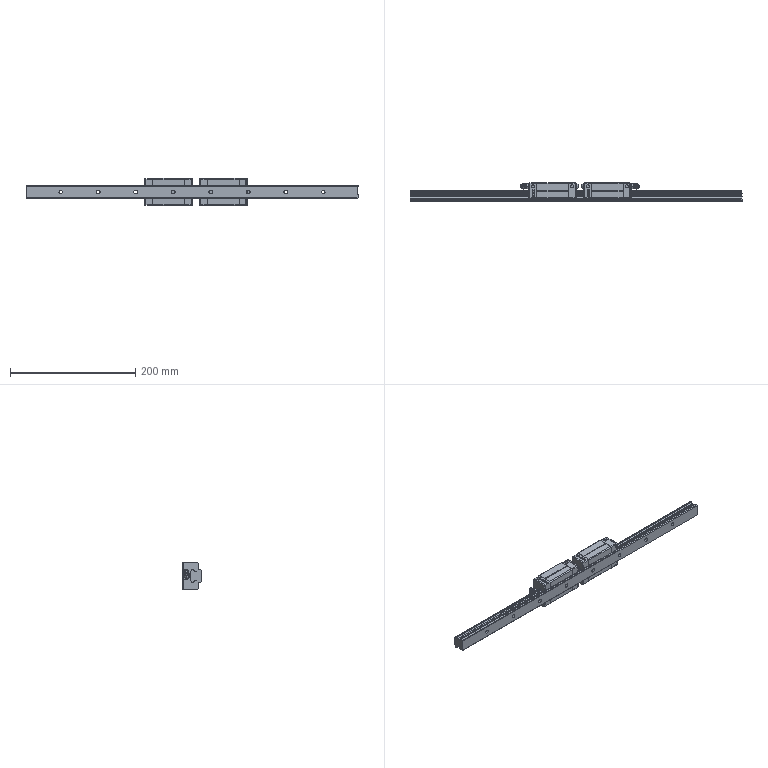Part | SolidWorks | 15 solids | 1721 faces | box 531 x 30 x 44 mm | volume 286413 mm3 | plane 1060 | cylinder 482 | cone 92 | spline 69 | sphere 12 | torus 6 | commonest cylinder face diameters 1 x148 0.2 x68 2 x58 4.06 x44 0.1 x36 6 x36